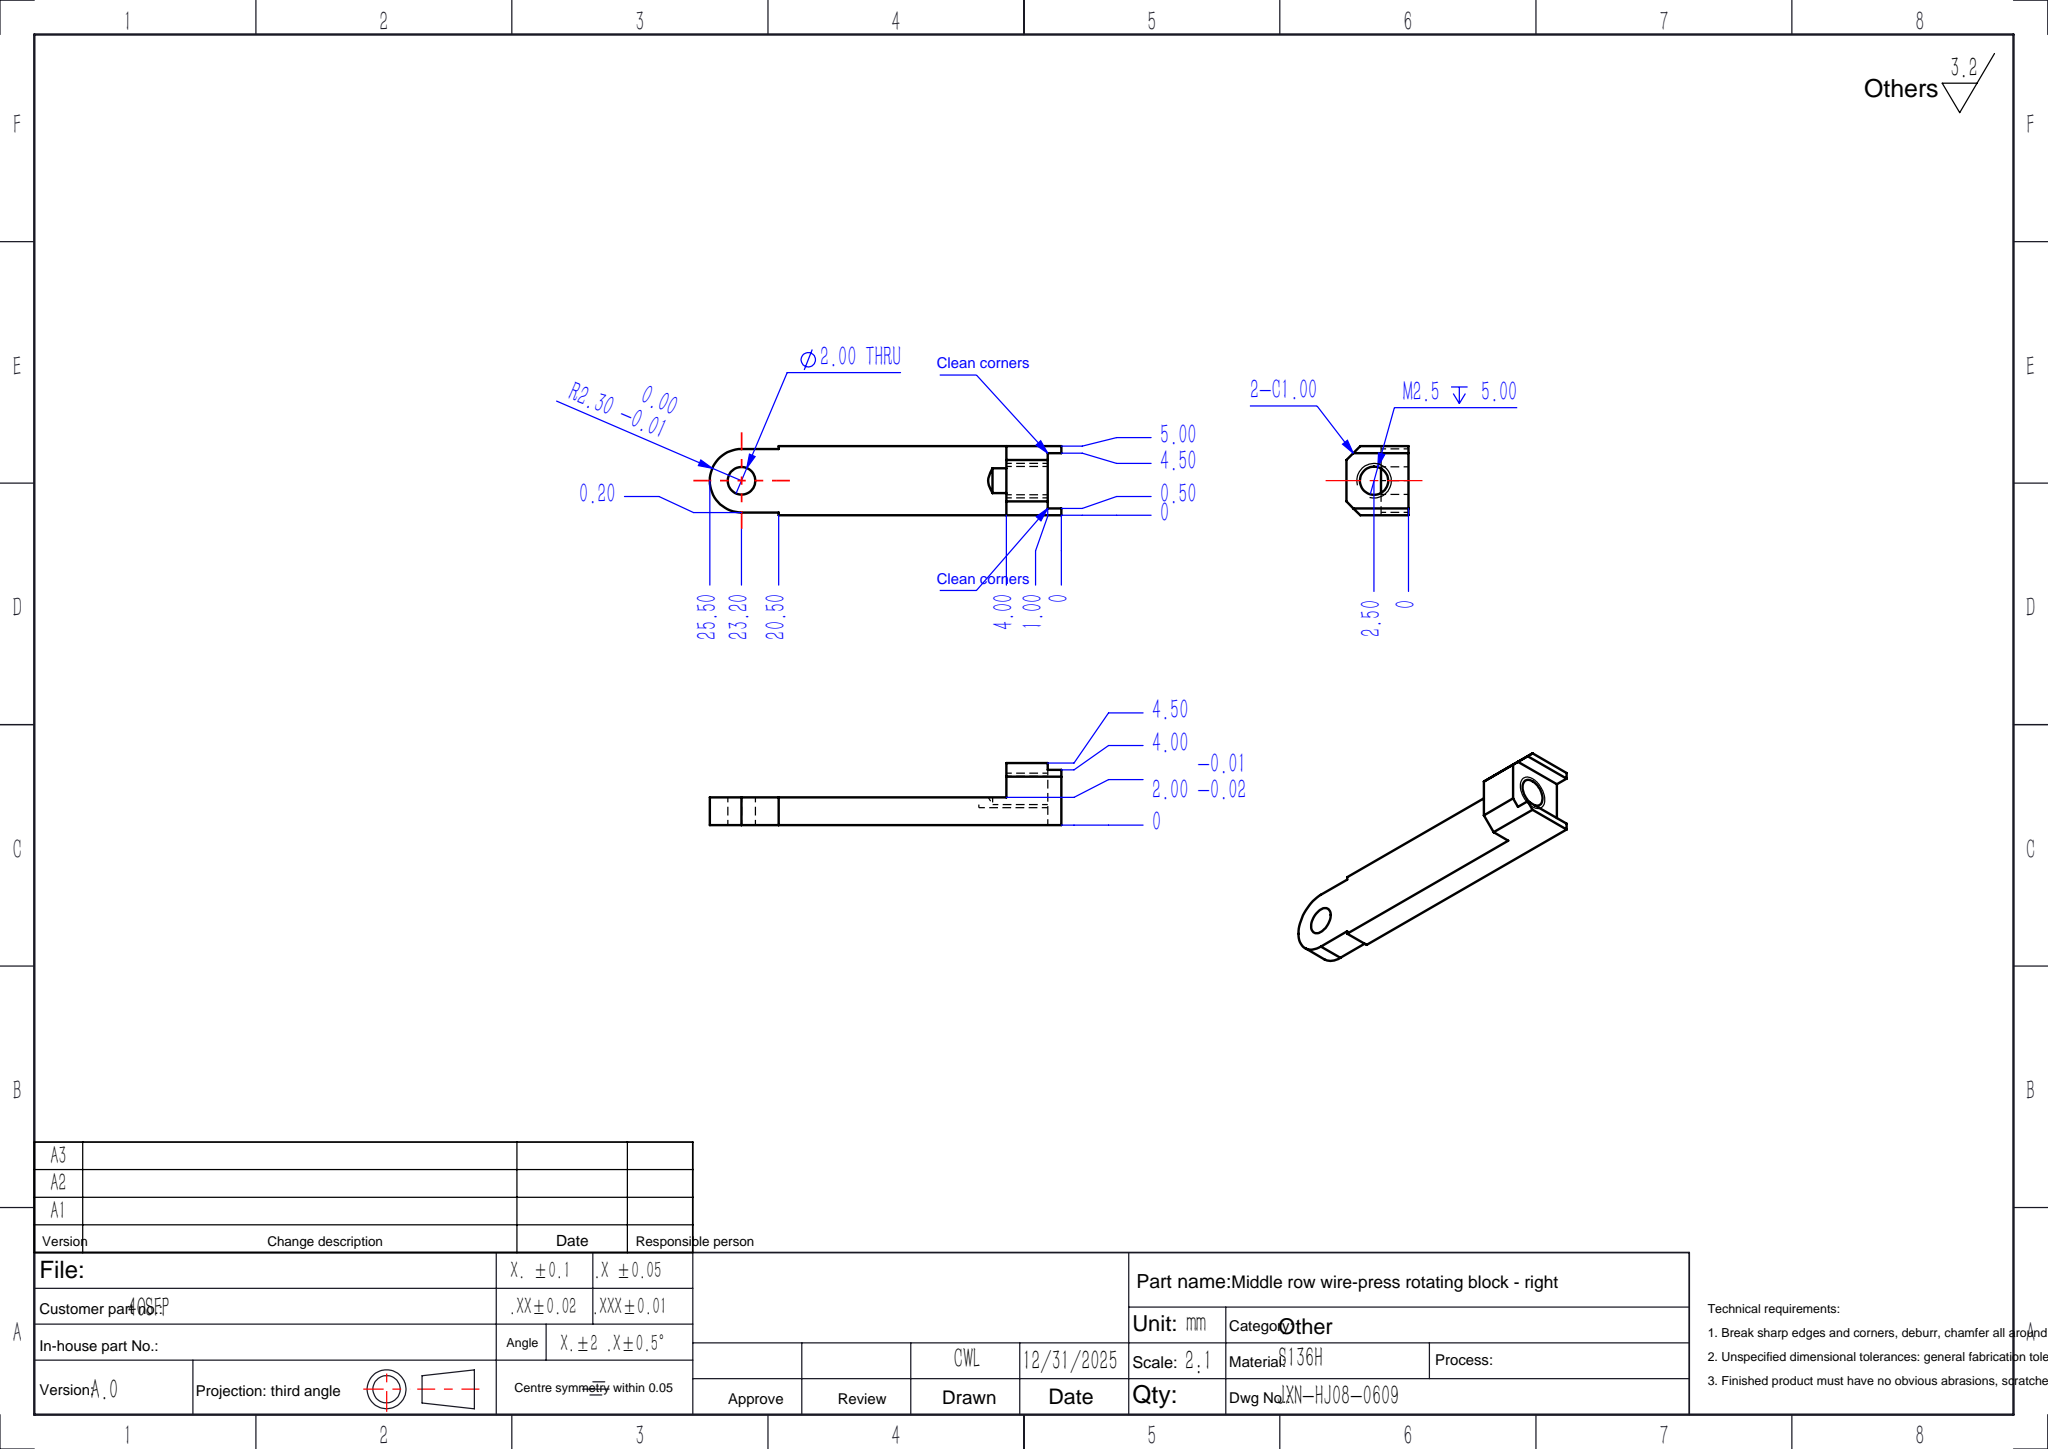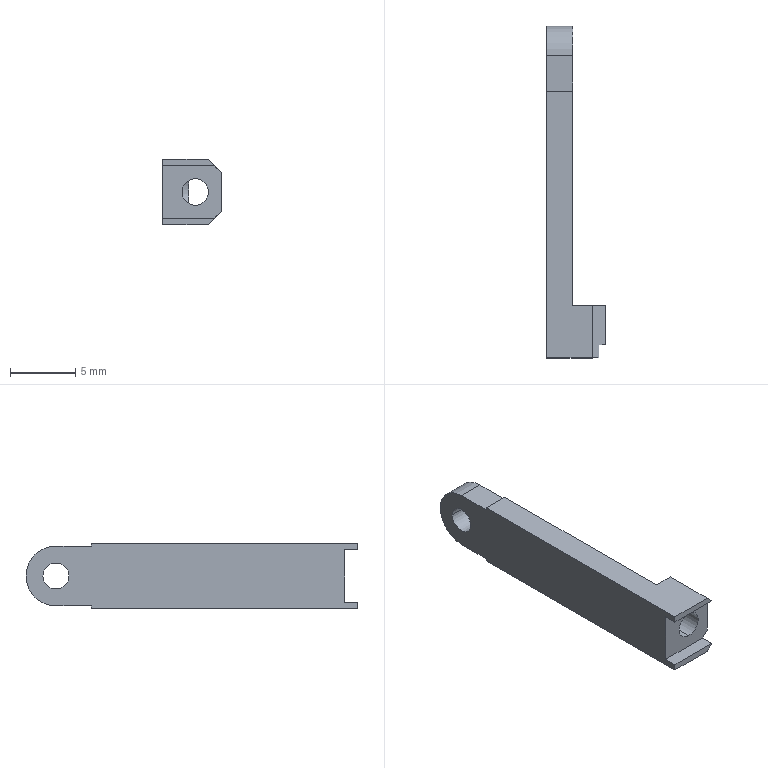Part | SolidWorks | features ICE 4, Chamfer 1, Extrusion 1, Fillet 1, HoleWzd 1 | 1 solid | 24 faces | box 4.5 x 25.5 x 5 mm | volume 257.777 mm3 | plane 17 | cylinder 6 | cone 1 | commonest cylinder face diameters 2 x2 2.05 x2 4.6 x2
STEP:
#1=CARTESIAN_POINT('',(2.5,-21.5,-1.475));
#2=VERTEX_POINT('',#1);
#3=CARTESIAN_POINT('',(2.,-21.5,-1.605));
#4=VERTEX_POINT('',#3);
#5=CARTESIAN_POINT('',(2.5,-21.5,-2.5));
#6=DIRECTION('',(0.,-1.,0.));
#7=DIRECTION('',(0.,0.,-1.));
#8=AXIS2_PLACEMENT_3D('',#5,#6,#7);
#9=CIRCLE('',#8,1.025);
#10=EDGE_CURVE('',#2,#4,#9,.T.);
#11=ORIENTED_EDGE('',*,*,#10,.F.);
#12=CARTESIAN_POINT('',(2.5,-24.5,-1.475));
#13=VERTEX_POINT('',#12);
#14=CARTESIAN_POINT('',(2.5,-24.5,-1.475));
#15=DIRECTION('',(0.,-1.,0.));
#16=VECTOR('',#15,1000.);
#17=LINE('',#14,#16);
#18=EDGE_CURVE('',#2,#13,#17,.T.);
#19=ORIENTED_EDGE('',*,*,#18,.T.);
#20=CARTESIAN_POINT('',(2.5,-24.5,-3.525));
#21=VERTEX_POINT('',#20);
#22=CARTESIAN_POINT('',(2.5,-24.5,-2.5));
#23=DIRECTION('',(0.,-1.,0.));
#24=DIRECTION('',(0.,0.,-1.));
#25=AXIS2_PLACEMENT_3D('',#22,#23,#24);
#26=CIRCLE('',#25,1.025);
#27=EDGE_CURVE('',#13,#21,#26,.T.);
#28=ORIENTED_EDGE('',*,*,#27,.T.);
#29=CARTESIAN_POINT('',(2.5,-21.5,-3.525));
#30=VERTEX_POINT('',#29);
#31=CARTESIAN_POINT('',(2.5,-24.5,-3.525));
#32=DIRECTION('',(0.,-1.,0.));
#33=VECTOR('',#32,1000.);
#34=LINE('',#31,#33);
#35=EDGE_CURVE('',#30,#21,#34,.T.);
#36=ORIENTED_EDGE('',*,*,#35,.F.);
#37=CARTESIAN_POINT('',(2.,-21.5,-3.395));
#38=VERTEX_POINT('',#37);
#39=CARTESIAN_POINT('',(2.5,-21.5,-2.5));
#40=DIRECTION('',(0.,-1.,0.));
#41=DIRECTION('',(0.,0.,-1.));
#42=AXIS2_PLACEMENT_3D('',#39,#40,#41);
#43=CIRCLE('',#42,1.025);
#44=EDGE_CURVE('',#38,#30,#43,.T.);
#45=ORIENTED_EDGE('',*,*,#44,.F.);
#46=CARTESIAN_POINT('',(2.,-20.5,-3.395));
#47=VERTEX_POINT('',#46);
#48=CARTESIAN_POINT('',(2.,-24.5,-3.395));
#49=DIRECTION('',(0.,-1.,0.));
#50=VECTOR('',#49,1000.);
#51=LINE('',#48,#50);
#52=EDGE_CURVE('',#47,#38,#51,.T.);
#53=ORIENTED_EDGE('',*,*,#52,.F.);
#54=CARTESIAN_POINT('',(2.,-20.5,-1.605));
#55=VERTEX_POINT('',#54);
#56=CARTESIAN_POINT('',(2.5,-20.5,-2.5));
#57=DIRECTION('',(0.,-1.,0.));
#58=DIRECTION('',(0.,0.,-1.));
#59=AXIS2_PLACEMENT_3D('',#56,#57,#58);
#60=CIRCLE('',#59,1.025);
#61=EDGE_CURVE('',#55,#47,#60,.T.);
#62=ORIENTED_EDGE('',*,*,#61,.F.);
#63=CARTESIAN_POINT('',(2.,-24.5,-1.605));
#64=DIRECTION('',(0.,1.,0.));
#65=VECTOR('',#64,1000.);
#66=LINE('',#63,#65);
#67=EDGE_CURVE('',#4,#55,#66,.T.);
#68=ORIENTED_EDGE('',*,*,#67,.F.);
#69=EDGE_LOOP('',(#11,#19,#28,#36,#45,#53,#62,#68));
#70=FACE_OUTER_BOUND('',#69,.T.);
#71=CARTESIAN_POINT('',(2.5,-24.5,-2.5));
#72=DIRECTION('',(0.,-1.,0.));
#73=DIRECTION('',(0.,0.,-1.));
#74=AXIS2_PLACEMENT_3D('',#71,#72,#73);
#75=CYLINDRICAL_SURFACE('',#74,1.025);
#76=ADVANCED_FACE('',(#70),#75,.F.);
#77=CARTESIAN_POINT('',(2.,-3.3,-2.5));
#78=VERTEX_POINT('',#77);
#79=CARTESIAN_POINT('',(2.,-1.3,-2.5));
#80=VERTEX_POINT('',#79);
#81=CARTESIAN_POINT('',(2.,-2.3,-2.5));
#82=DIRECTION('',(1.,0.,0.));
#83=DIRECTION('',(0.,-1.,0.));
#84=AXIS2_PLACEMENT_3D('',#81,#82,#83);
#85=CIRCLE('',#84,1.);
#86=EDGE_CURVE('',#78,#80,#85,.T.);
#87=ORIENTED_EDGE('',*,*,#86,.T.);
#88=CARTESIAN_POINT('',(0.,-1.3,-2.5));
#89=VERTEX_POINT('',#88);
#90=CARTESIAN_POINT('',(4.5,-1.3,-2.5));
#91=DIRECTION('',(-1.,0.,0.));
#92=VECTOR('',#91,1000.);
#93=LINE('',#90,#92);
#94=EDGE_CURVE('',#80,#89,#93,.T.);
#95=ORIENTED_EDGE('',*,*,#94,.T.);
#96=CARTESIAN_POINT('',(0.,-3.3,-2.5));
#97=VERTEX_POINT('',#96);
#98=CARTESIAN_POINT('',(0.,-2.3,-2.5));
#99=DIRECTION('',(-1.,0.,0.));
#100=DIRECTION('',(0.,-1.,0.));
#101=AXIS2_PLACEMENT_3D('',#98,#99,#100);
#102=CIRCLE('',#101,1.);
#103=EDGE_CURVE('',#89,#97,#102,.T.);
#104=ORIENTED_EDGE('',*,*,#103,.T.);
#105=CARTESIAN_POINT('',(4.5,-3.3,-2.5));
#106=DIRECTION('',(-1.,0.,0.));
#107=VECTOR('',#106,1000.);
#108=LINE('',#105,#107);
#109=EDGE_CURVE('',#78,#97,#108,.T.);
#110=ORIENTED_EDGE('',*,*,#109,.F.);
#111=EDGE_LOOP('',(#87,#95,#104,#110));
#112=FACE_OUTER_BOUND('',#111,.T.);
#113=CARTESIAN_POINT('',(4.5,-2.3,-2.5));
#114=DIRECTION('',(-1.,0.,0.));
#115=DIRECTION('',(0.,-1.,0.));
#116=AXIS2_PLACEMENT_3D('',#113,#114,#115);
#117=CYLINDRICAL_SURFACE('',#116,1.);
#118=ADVANCED_FACE('',(#112),#117,.F.);
#119=CARTESIAN_POINT('',(4.,-25.5,-0.5));
#120=VERTEX_POINT('',#119);
#121=CARTESIAN_POINT('',(0.,-25.5,-0.5));
#122=VERTEX_POINT('',#121);
#123=CARTESIAN_POINT('',(4.5,-25.5,-0.5));
#124=DIRECTION('',(-1.,0.,0.));
#125=VECTOR('',#124,1000.);
#126=LINE('',#123,#125);
#127=EDGE_CURVE('',#120,#122,#126,.T.);
#128=ORIENTED_EDGE('',*,*,#127,.F.);
#129=CARTESIAN_POINT('',(3.5,-25.5,0.));
#130=VERTEX_POINT('',#129);
#131=CARTESIAN_POINT('',(4.25,-25.5,-0.75));
#132=DIRECTION('',(-0.7071,0.,0.7071));
#133=VECTOR('',#132,1000.);
#134=LINE('',#131,#133);
#135=EDGE_CURVE('',#120,#130,#134,.T.);
#136=ORIENTED_EDGE('',*,*,#135,.T.);
#137=CARTESIAN_POINT('',(0.,-25.5,0.));
#138=VERTEX_POINT('',#137);
#139=CARTESIAN_POINT('',(0.,-25.5,0.));
#140=DIRECTION('',(1.,0.,0.));
#141=VECTOR('',#140,1000.);
#142=LINE('',#139,#141);
#143=EDGE_CURVE('',#138,#130,#142,.T.);
#144=ORIENTED_EDGE('',*,*,#143,.F.);
#145=CARTESIAN_POINT('',(0.,-25.5,-5.));
#146=DIRECTION('',(0.,0.,1.));
#147=VECTOR('',#146,1000.);
#148=LINE('',#145,#147);
#149=EDGE_CURVE('',#122,#138,#148,.T.);
#150=ORIENTED_EDGE('',*,*,#149,.F.);
#151=EDGE_LOOP('',(#128,#136,#144,#150));
#152=FACE_OUTER_BOUND('',#151,.T.);
#153=CARTESIAN_POINT('',(0.,-25.5,-5.));
#154=DIRECTION('',(0.,-1.,0.));
#155=DIRECTION('',(0.,0.,-1.));
#156=AXIS2_PLACEMENT_3D('',#153,#154,#155);
#157=PLANE('',#156);
#158=ADVANCED_FACE('',(#152),#157,.T.);
#159=CARTESIAN_POINT('',(0.,-24.5,-0.5));
#160=VERTEX_POINT('',#159);
#161=CARTESIAN_POINT('',(0.,-25.5,-0.5));
#162=DIRECTION('',(0.,1.,0.));
#163=VECTOR('',#162,1000.);
#164=LINE('',#161,#163);
#165=EDGE_CURVE('',#122,#160,#164,.T.);
#166=ORIENTED_EDGE('',*,*,#165,.F.);
#167=ORIENTED_EDGE('',*,*,#149,.T.);
#168=CARTESIAN_POINT('',(0.,-5.,0.));
#169=VERTEX_POINT('',#168);
#170=CARTESIAN_POINT('',(0.,0.,0.));
#171=DIRECTION('',(0.,-1.,0.));
#172=VECTOR('',#171,1000.);
#173=LINE('',#170,#172);
#174=EDGE_CURVE('',#169,#138,#173,.T.);
#175=ORIENTED_EDGE('',*,*,#174,.F.);
#176=CARTESIAN_POINT('',(0.,-5.,-0.2));
#177=VERTEX_POINT('',#176);
#178=CARTESIAN_POINT('',(0.,-5.,0.));
#179=DIRECTION('',(0.,0.,1.));
#180=VECTOR('',#179,1000.);
#181=LINE('',#178,#180);
#182=EDGE_CURVE('',#177,#169,#181,.T.);
#183=ORIENTED_EDGE('',*,*,#182,.F.);
#184=CARTESIAN_POINT('',(0.,-2.3,-0.2));
#185=VERTEX_POINT('',#184);
#186=CARTESIAN_POINT('',(0.,0.,-0.2));
#187=DIRECTION('',(0.,-1.,0.));
#188=VECTOR('',#187,1000.);
#189=LINE('',#186,#188);
#190=EDGE_CURVE('',#185,#177,#189,.T.);
#191=ORIENTED_EDGE('',*,*,#190,.F.);
#192=CARTESIAN_POINT('',(0.,0.,-2.5));
#193=VERTEX_POINT('',#192);
#194=CARTESIAN_POINT('',(0.,-2.3,-2.5));
#195=DIRECTION('',(-1.,0.,0.));
#196=DIRECTION('',(0.,-1.,0.));
#197=AXIS2_PLACEMENT_3D('',#194,#195,#196);
#198=CIRCLE('',#197,2.3);
#199=EDGE_CURVE('',#185,#193,#198,.T.);
#200=ORIENTED_EDGE('',*,*,#199,.T.);
#201=CARTESIAN_POINT('',(0.,-2.3,-4.8));
#202=VERTEX_POINT('',#201);
#203=CARTESIAN_POINT('',(0.,-2.3,-2.5));
#204=DIRECTION('',(-1.,0.,0.));
#205=DIRECTION('',(0.,-1.,0.));
#206=AXIS2_PLACEMENT_3D('',#203,#204,#205);
#207=CIRCLE('',#206,2.3);
#208=EDGE_CURVE('',#193,#202,#207,.T.);
#209=ORIENTED_EDGE('',*,*,#208,.T.);
#210=CARTESIAN_POINT('',(0.,-5.,-4.8));
#211=VERTEX_POINT('',#210);
#212=CARTESIAN_POINT('',(0.,0.,-4.8));
#213=DIRECTION('',(0.,1.,0.));
#214=VECTOR('',#213,1000.);
#215=LINE('',#212,#214);
#216=EDGE_CURVE('',#211,#202,#215,.T.);
#217=ORIENTED_EDGE('',*,*,#216,.F.);
#218=CARTESIAN_POINT('',(0.,-5.,-5.));
#219=VERTEX_POINT('',#218);
#220=CARTESIAN_POINT('',(0.,-5.,-5.));
#221=DIRECTION('',(0.,0.,1.));
#222=VECTOR('',#221,1000.);
#223=LINE('',#220,#222);
#224=EDGE_CURVE('',#219,#211,#223,.T.);
#225=ORIENTED_EDGE('',*,*,#224,.F.);
#226=CARTESIAN_POINT('',(0.,-25.5,-5.));
#227=VERTEX_POINT('',#226);
#228=CARTESIAN_POINT('',(0.,0.,-5.));
#229=DIRECTION('',(0.,-1.,0.));
#230=VECTOR('',#229,1000.);
#231=LINE('',#228,#230);
#232=EDGE_CURVE('',#219,#227,#231,.T.);
#233=ORIENTED_EDGE('',*,*,#232,.T.);
#234=CARTESIAN_POINT('',(0.,-25.5,-4.5));
#235=VERTEX_POINT('',#234);
#236=CARTESIAN_POINT('',(0.,-25.5,-5.));
#237=DIRECTION('',(0.,0.,1.));
#238=VECTOR('',#237,1000.);
#239=LINE('',#236,#238);
#240=EDGE_CURVE('',#227,#235,#239,.T.);
#241=ORIENTED_EDGE('',*,*,#240,.T.);
#242=CARTESIAN_POINT('',(0.,-24.5,-4.5));
#243=VERTEX_POINT('',#242);
#244=CARTESIAN_POINT('',(0.,-25.5,-4.5));
#245=DIRECTION('',(0.,-1.,0.));
#246=VECTOR('',#245,1000.);
#247=LINE('',#244,#246);
#248=EDGE_CURVE('',#243,#235,#247,.T.);
#249=ORIENTED_EDGE('',*,*,#248,.F.);
#250=CARTESIAN_POINT('',(0.,-24.5,-0.5));
#251=DIRECTION('',(0.,0.,-1.));
#252=VECTOR('',#251,1000.);
#253=LINE('',#250,#252);
#254=EDGE_CURVE('',#160,#243,#253,.T.);
#255=ORIENTED_EDGE('',*,*,#254,.F.);
#256=EDGE_LOOP('',(#166,#167,#175,#183,#191,#200,#209,#217,#225,#233,#241,#249,#255));
#257=FACE_OUTER_BOUND('',#256,.T.);
#258=CARTESIAN_POINT('',(0.,-2.3,-2.5));
#259=DIRECTION('',(-1.,0.,0.));
#260=DIRECTION('',(0.,-1.,0.));
#261=AXIS2_PLACEMENT_3D('',#258,#259,#260);
#262=CIRCLE('',#261,1.);
#263=EDGE_CURVE('',#97,#89,#262,.T.);
#264=ORIENTED_EDGE('',*,*,#263,.F.);
#265=ORIENTED_EDGE('',*,*,#103,.F.);
#266=EDGE_LOOP('',(#264,#265));
#267=FACE_BOUND('',#266,.T.);
#268=CARTESIAN_POINT('',(0.,0.,-5.));
#269=DIRECTION('',(-1.,0.,0.));
#270=DIRECTION('',(0.,-1.,0.));
#271=AXIS2_PLACEMENT_3D('',#268,#269,#270);
#272=PLANE('',#271);
#273=ADVANCED_FACE('',(#257,#267),#272,.T.);
#274=CARTESIAN_POINT('',(4.5,-21.5,-4.));
#275=VERTEX_POINT('',#274);
#276=CARTESIAN_POINT('',(4.5,-21.5,-1.));
#277=VERTEX_POINT('',#276);
#278=CARTESIAN_POINT('',(4.5,-21.5,-5.));
#279=DIRECTION('',(0.,0.,1.));
#280=VECTOR('',#279,1000.);
#281=LINE('',#278,#280);
#282=EDGE_CURVE('',#275,#277,#281,.T.);
#283=ORIENTED_EDGE('',*,*,#282,.T.);
#284=CARTESIAN_POINT('',(4.5,-24.5,-1.));
#285=VERTEX_POINT('',#284);
#286=CARTESIAN_POINT('',(4.5,0.,-1.));
#287=DIRECTION('',(0.,-1.,0.));
#288=VECTOR('',#287,1000.);
#289=LINE('',#286,#288);
#290=EDGE_CURVE('',#277,#285,#289,.T.);
#291=ORIENTED_EDGE('',*,*,#290,.T.);
#292=CARTESIAN_POINT('',(4.5,-24.5,-4.));
#293=VERTEX_POINT('',#292);
#294=CARTESIAN_POINT('',(4.5,-24.5,-0.5));
#295=DIRECTION('',(0.,0.,-1.));
#296=VECTOR('',#295,1000.);
#297=LINE('',#294,#296);
#298=EDGE_CURVE('',#285,#293,#297,.T.);
#299=ORIENTED_EDGE('',*,*,#298,.T.);
#300=CARTESIAN_POINT('',(4.5,-21.5,-4.));
#301=DIRECTION('',(0.,1.,0.));
#302=VECTOR('',#301,1000.);
#303=LINE('',#300,#302);
#304=EDGE_CURVE('',#293,#275,#303,.T.);
#305=ORIENTED_EDGE('',*,*,#304,.T.);
#306=EDGE_LOOP('',(#283,#291,#299,#305));
#307=FACE_OUTER_BOUND('',#306,.T.);
#308=CARTESIAN_POINT('',(4.5,0.,-5.));
#309=DIRECTION('',(1.,0.,0.));
#310=DIRECTION('',(0.,1.,0.));
#311=AXIS2_PLACEMENT_3D('',#308,#309,#310);
#312=PLANE('',#311);
#313=ADVANCED_FACE('',(#307),#312,.T.);
#314=CARTESIAN_POINT('',(3.5,-25.5,-5.));
#315=VERTEX_POINT('',#314);
#316=CARTESIAN_POINT('',(0.,-25.5,-5.));
#317=DIRECTION('',(1.,0.,0.));
#318=VECTOR('',#317,1000.);
#319=LINE('',#316,#318);
#320=EDGE_CURVE('',#227,#315,#319,.T.);
#321=ORIENTED_EDGE('',*,*,#320,.T.);
#322=CARTESIAN_POINT('',(4.,-25.5,-4.5));
#323=VERTEX_POINT('',#322);
#324=CARTESIAN_POINT('',(1.75,-25.5,-6.75));
#325=DIRECTION('',(0.7071,0.,0.7071));
#326=VECTOR('',#325,1000.);
#327=LINE('',#324,#326);
#328=EDGE_CURVE('',#315,#323,#327,.T.);
#329=ORIENTED_EDGE('',*,*,#328,.T.);
#330=CARTESIAN_POINT('',(4.5,-25.5,-4.5));
#331=DIRECTION('',(-1.,0.,0.));
#332=VECTOR('',#331,1000.);
#333=LINE('',#330,#332);
#334=EDGE_CURVE('',#323,#235,#333,.T.);
#335=ORIENTED_EDGE('',*,*,#334,.T.);
#336=ORIENTED_EDGE('',*,*,#240,.F.);
#337=EDGE_LOOP('',(#321,#329,#335,#336));
#338=FACE_OUTER_BOUND('',#337,.T.);
#339=CARTESIAN_POINT('',(0.,-25.5,-5.));
#340=DIRECTION('',(0.,-1.,0.));
#341=DIRECTION('',(0.,0.,-1.));
#342=AXIS2_PLACEMENT_3D('',#339,#340,#341);
#343=PLANE('',#342);
#344=ADVANCED_FACE('',(#338),#343,.T.);
#345=CARTESIAN_POINT('',(2.,-21.5,-5.));
#346=VERTEX_POINT('',#345);
#347=CARTESIAN_POINT('',(3.5,-21.5,-5.));
#348=VERTEX_POINT('',#347);
#349=CARTESIAN_POINT('',(4.5,-21.5,-5.));
#350=DIRECTION('',(1.,0.,0.));
#351=VECTOR('',#350,1000.);
#352=LINE('',#349,#351);
#353=EDGE_CURVE('',#346,#348,#352,.T.);
#354=ORIENTED_EDGE('',*,*,#353,.T.);
#355=CARTESIAN_POINT('',(3.5,-25.5,-5.));
#356=DIRECTION('',(0.,-1.,0.));
#357=VECTOR('',#356,1000.);
#358=LINE('',#355,#357);
#359=EDGE_CURVE('',#348,#315,#358,.T.);
#360=ORIENTED_EDGE('',*,*,#359,.T.);
#361=ORIENTED_EDGE('',*,*,#320,.F.);
#362=ORIENTED_EDGE('',*,*,#232,.F.);
#363=CARTESIAN_POINT('',(2.,-5.,-5.));
#364=VERTEX_POINT('',#363);
#365=CARTESIAN_POINT('',(4.5,-5.,-5.));
#366=DIRECTION('',(-1.,0.,0.));
#367=VECTOR('',#366,1000.);
#368=LINE('',#365,#367);
#369=EDGE_CURVE('',#364,#219,#368,.T.);
#370=ORIENTED_EDGE('',*,*,#369,.F.);
#371=CARTESIAN_POINT('',(2.,0.,-5.));
#372=DIRECTION('',(0.,-1.,0.));
#373=VECTOR('',#372,1000.);
#374=LINE('',#371,#373);
#375=EDGE_CURVE('',#364,#346,#374,.T.);
#376=ORIENTED_EDGE('',*,*,#375,.T.);
#377=EDGE_LOOP('',(#354,#360,#361,#362,#370,#376));
#378=FACE_OUTER_BOUND('',#377,.T.);
#379=CARTESIAN_POINT('',(0.,0.,-5.));
#380=DIRECTION('',(0.,0.,1.));
#381=DIRECTION('',(1.,0.,0.));
#382=AXIS2_PLACEMENT_3D('',#379,#380,#381);
#383=PLANE('',#382);
#384=ADVANCED_FACE('',(#378),#383,.F.);
#385=ORIENTED_EDGE('',*,*,#143,.T.);
#386=CARTESIAN_POINT('',(3.5,-21.5,0.));
#387=VERTEX_POINT('',#386);
#388=CARTESIAN_POINT('',(3.5,0.,0.));
#389=DIRECTION('',(0.,1.,0.));
#390=VECTOR('',#389,1000.);
#391=LINE('',#388,#390);
#392=EDGE_CURVE('',#130,#387,#391,.T.);
#393=ORIENTED_EDGE('',*,*,#392,.T.);
#394=CARTESIAN_POINT('',(2.,-21.5,0.));
#395=VERTEX_POINT('',#394);
#396=CARTESIAN_POINT('',(4.5,-21.5,0.));
#397=DIRECTION('',(1.,0.,0.));
#398=VECTOR('',#397,1000.);
#399=LINE('',#396,#398);
#400=EDGE_CURVE('',#395,#387,#399,.T.);
#401=ORIENTED_EDGE('',*,*,#400,.F.);
#402=CARTESIAN_POINT('',(2.,-5.,0.));
#403=VERTEX_POINT('',#402);
#404=CARTESIAN_POINT('',(2.,0.,0.));
#405=DIRECTION('',(0.,-1.,0.));
#406=VECTOR('',#405,1000.);
#407=LINE('',#404,#406);
#408=EDGE_CURVE('',#403,#395,#407,.T.);
#409=ORIENTED_EDGE('',*,*,#408,.F.);
#410=CARTESIAN_POINT('',(4.5,-5.,0.));
#411=DIRECTION('',(-1.,0.,0.));
#412=VECTOR('',#411,1000.);
#413=LINE('',#410,#412);
#414=EDGE_CURVE('',#403,#169,#413,.T.);
#415=ORIENTED_EDGE('',*,*,#414,.T.);
#416=ORIENTED_EDGE('',*,*,#174,.T.);
#417=EDGE_LOOP('',(#385,#393,#401,#409,#415,#416));
#418=FACE_OUTER_BOUND('',#417,.T.);
#419=CARTESIAN_POINT('',(0.,0.,0.));
#420=DIRECTION('',(0.,0.,1.));
#421=DIRECTION('',(1.,0.,0.));
#422=AXIS2_PLACEMENT_3D('',#419,#420,#421);
#423=PLANE('',#422);
#424=ADVANCED_FACE('',(#418),#423,.T.);
#425=ORIENTED_EDGE('',*,*,#94,.F.);
#426=CARTESIAN_POINT('',(2.,-2.3,-2.5));
#427=DIRECTION('',(1.,0.,0.));
#428=DIRECTION('',(0.,-1.,0.));
#429=AXIS2_PLACEMENT_3D('',#426,#427,#428);
#430=CIRCLE('',#429,1.);
#431=EDGE_CURVE('',#80,#78,#430,.T.);
#432=ORIENTED_EDGE('',*,*,#431,.T.);
#433=ORIENTED_EDGE('',*,*,#109,.T.);
#434=ORIENTED_EDGE('',*,*,#263,.T.);
#435=EDGE_LOOP('',(#425,#432,#433,#434));
#436=FACE_OUTER_BOUND('',#435,.T.);
#437=CARTESIAN_POINT('',(4.5,-2.3,-2.5));
#438=DIRECTION('',(-1.,0.,0.));
#439=DIRECTION('',(0.,-1.,0.));
#440=AXIS2_PLACEMENT_3D('',#437,#438,#439);
#441=CYLINDRICAL_SURFACE('',#440,1.);
#442=ADVANCED_FACE('',(#436),#441,.F.);
#443=ORIENTED_EDGE('',*,*,#414,.F.);
#444=CARTESIAN_POINT('',(2.,-5.,-0.2));
#445=VERTEX_POINT('',#444);
#446=CARTESIAN_POINT('',(2.,-5.,0.));
#447=DIRECTION('',(0.,0.,-1.));
#448=VECTOR('',#447,1000.);
#449=LINE('',#446,#448);
#450=EDGE_CURVE('',#403,#445,#449,.T.);
#451=ORIENTED_EDGE('',*,*,#450,.T.);
#452=CARTESIAN_POINT('',(4.5,-5.,-0.2));
#453=DIRECTION('',(-1.,0.,0.));
#454=VECTOR('',#453,1000.);
#455=LINE('',#452,#454);
#456=EDGE_CURVE('',#445,#177,#455,.T.);
#457=ORIENTED_EDGE('',*,*,#456,.T.);
#458=ORIENTED_EDGE('',*,*,#182,.T.);
#459=EDGE_LOOP('',(#443,#451,#457,#458));
#460=FACE_OUTER_BOUND('',#459,.T.);
#461=CARTESIAN_POINT('',(4.5,-5.,0.));
#462=DIRECTION('',(0.,-1.,0.));
#463=DIRECTION('',(1.,0.,0.));
#464=AXIS2_PLACEMENT_3D('',#461,#462,#463);
#465=PLANE('',#464);
#466=ADVANCED_FACE('',(#460),#465,.F.);
#467=ORIENTED_EDGE('',*,*,#456,.F.);
#468=CARTESIAN_POINT('',(2.,-2.3,-0.2));
#469=VERTEX_POINT('',#468);
#470=CARTESIAN_POINT('',(2.,0.,-0.2));
#471=DIRECTION('',(0.,1.,0.));
#472=VECTOR('',#471,1000.);
#473=LINE('',#470,#472);
#474=EDGE_CURVE('',#445,#469,#473,.T.);
#475=ORIENTED_EDGE('',*,*,#474,.T.);
#476=CARTESIAN_POINT('',(0.,-2.3,-0.2));
#477=DIRECTION('',(-1.,0.,0.));
#478=VECTOR('',#477,1000.);
#479=LINE('',#476,#478);
#480=EDGE_CURVE('',#469,#185,#479,.T.);
#481=ORIENTED_EDGE('',*,*,#480,.T.);
#482=ORIENTED_EDGE('',*,*,#190,.T.);
#483=EDGE_LOOP('',(#467,#475,#481,#482));
#484=FACE_OUTER_BOUND('',#483,.T.);
#485=CARTESIAN_POINT('',(4.5,0.,-0.2));
#486=DIRECTION('',(0.,0.,-1.));
#487=DIRECTION('',(0.,1.,0.));
#488=AXIS2_PLACEMENT_3D('',#485,#486,#487);
#489=PLANE('',#488);
#490=ADVANCED_FACE('',(#484),#489,.F.);
#491=CARTESIAN_POINT('',(2.,-2.3,-4.8));
#492=VERTEX_POINT('',#491);
#493=CARTESIAN_POINT('',(4.5,-2.3,-4.8));
#494=DIRECTION('',(1.,0.,0.));
#495=VECTOR('',#494,1000.);
#496=LINE('',#493,#495);
#497=EDGE_CURVE('',#202,#492,#496,.T.);
#498=ORIENTED_EDGE('',*,*,#497,.T.);
#499=CARTESIAN_POINT('',(2.,-5.,-4.8));
#500=VERTEX_POINT('',#499);
#501=CARTESIAN_POINT('',(2.,0.,-4.8));
#502=DIRECTION('',(0.,-1.,0.));
#503=VECTOR('',#502,1000.);
#504=LINE('',#501,#503);
#505=EDGE_CURVE('',#492,#500,#504,.T.);
#506=ORIENTED_EDGE('',*,*,#505,.T.);
#507=CARTESIAN_POINT('',(4.5,-5.,-4.8));
#508=DIRECTION('',(-1.,0.,0.));
#509=VECTOR('',#508,1000.);
#510=LINE('',#507,#509);
#511=EDGE_CURVE('',#500,#211,#510,.T.);
#512=ORIENTED_EDGE('',*,*,#511,.T.);
#513=ORIENTED_EDGE('',*,*,#216,.T.);
#514=EDGE_LOOP('',(#498,#506,#512,#513));
#515=FACE_OUTER_BOUND('',#514,.T.);
#516=CARTESIAN_POINT('',(4.5,0.,-4.8));
#517=DIRECTION('',(0.,0.,1.));
#518=DIRECTION('',(0.,-1.,0.));
#519=AXIS2_PLACEMENT_3D('',#516,#517,#518);
#520=PLANE('',#519);
#521=ADVANCED_FACE('',(#515),#520,.F.);
#522=ORIENTED_EDGE('',*,*,#511,.F.);
#523=CARTESIAN_POINT('',(2.,-5.,-5.));
#524=DIRECTION('',(0.,0.,-1.));
#525=VECTOR('',#524,1000.);
#526=LINE('',#523,#525);
#527=EDGE_CURVE('',#500,#364,#526,.T.);
#528=ORIENTED_EDGE('',*,*,#527,.T.);
#529=ORIENTED_EDGE('',*,*,#369,.T.);
#530=ORIENTED_EDGE('',*,*,#224,.T.);
#531=EDGE_LOOP('',(#522,#528,#529,#530));
#532=FACE_OUTER_BOUND('',#531,.T.);
#533=CARTESIAN_POINT('',(4.5,-5.,-5.));
#534=DIRECTION('',(0.,-1.,0.));
#535=DIRECTION('',(1.,0.,0.));
#536=AXIS2_PLACEMENT_3D('',#533,#534,#535);
#537=PLANE('',#536);
#538=ADVANCED_FACE('',(#532),#537,.F.);
#539=CARTESIAN_POINT('',(2.,0.,-2.5));
#540=VERTEX_POINT('',#539);
#541=CARTESIAN_POINT('',(2.,-2.3,-2.5));
#542=DIRECTION('',(1.,0.,0.));
#543=DIRECTION('',(0.,-1.,0.));
#544=AXIS2_PLACEMENT_3D('',#541,#542,#543);
#545=CIRCLE('',#544,2.3);
#546=EDGE_CURVE('',#540,#469,#545,.T.);
#547=ORIENTED_EDGE('',*,*,#546,.F.);
#548=CARTESIAN_POINT('',(4.5,0.,-2.5));
#549=DIRECTION('',(1.,0.,0.));
#550=VECTOR('',#549,1000.);
#551=LINE('',#548,#550);
#552=EDGE_CURVE('',#193,#540,#551,.T.);
#553=ORIENTED_EDGE('',*,*,#552,.F.);
#554=ORIENTED_EDGE('',*,*,#199,.F.);
#555=ORIENTED_EDGE('',*,*,#480,.F.);
#556=EDGE_LOOP('',(#547,#553,#554,#555));
#557=FACE_OUTER_BOUND('',#556,.T.);
#558=CARTESIAN_POINT('',(4.5,-2.3,-2.5));
#559=DIRECTION('',(1.,0.,0.));
#560=DIRECTION('',(0.,0.,-1.));
#561=AXIS2_PLACEMENT_3D('',#558,#559,#560);
#562=CYLINDRICAL_SURFACE('',#561,2.3);
#563=ADVANCED_FACE('',(#557),#562,.T.);
#564=CARTESIAN_POINT('',(2.,-2.3,-2.5));
#565=DIRECTION('',(1.,0.,0.));
#566=DIRECTION('',(0.,-1.,0.));
#567=AXIS2_PLACEMENT_3D('',#564,#565,#566);
#568=CIRCLE('',#567,2.3);
#569=EDGE_CURVE('',#492,#540,#568,.T.);
#570=ORIENTED_EDGE('',*,*,#569,.F.);
#571=ORIENTED_EDGE('',*,*,#497,.F.);
#572=ORIENTED_EDGE('',*,*,#208,.F.);
#573=ORIENTED_EDGE('',*,*,#552,.T.);
#574=EDGE_LOOP('',(#570,#571,#572,#573));
#575=FACE_OUTER_BOUND('',#574,.T.);
#576=CARTESIAN_POINT('',(0.,-2.3,-2.5));
#577=DIRECTION('',(1.,0.,0.));
#578=DIRECTION('',(0.,0.,-1.));
#579=AXIS2_PLACEMENT_3D('',#576,#577,#578);
#580=CYLINDRICAL_SURFACE('',#579,2.3);
#581=ADVANCED_FACE('',(#575),#580,.T.);
#582=CARTESIAN_POINT('',(4.,-24.5,-0.5));
#583=VERTEX_POINT('',#582);
#584=CARTESIAN_POINT('',(4.5,-24.5,-0.5));
#585=DIRECTION('',(-1.,0.,0.));
#586=VECTOR('',#585,1000.);
#587=LINE('',#584,#586);
#588=EDGE_CURVE('',#583,#160,#587,.T.);
#589=ORIENTED_EDGE('',*,*,#588,.F.);
#590=CARTESIAN_POINT('',(4.,0.,-0.5));
#591=DIRECTION('',(0.,-1.,0.));
#592=VECTOR('',#591,1000.);
#593=LINE('',#590,#592);
#594=EDGE_CURVE('',#583,#120,#593,.T.);
#595=ORIENTED_EDGE('',*,*,#594,.T.);
#596=ORIENTED_EDGE('',*,*,#127,.T.);
#597=ORIENTED_EDGE('',*,*,#165,.T.);
#598=EDGE_LOOP('',(#589,#595,#596,#597));
#599=FACE_OUTER_BOUND('',#598,.T.);
#600=CARTESIAN_POINT('',(4.5,-25.5,-0.5));
#601=DIRECTION('',(0.,0.,1.));
#602=DIRECTION('',(0.,-1.,0.));
#603=AXIS2_PLACEMENT_3D('',#600,#601,#602);
#604=PLANE('',#603);
#605=ADVANCED_FACE('',(#599),#604,.F.);
#606=ORIENTED_EDGE('',*,*,#334,.F.);
#607=CARTESIAN_POINT('',(4.,-24.5,-4.5));
#608=VERTEX_POINT('',#607);
#609=CARTESIAN_POINT('',(4.,0.,-4.5));
#610=DIRECTION('',(0.,1.,0.));
#611=VECTOR('',#610,1000.);
#612=LINE('',#609,#611);
#613=EDGE_CURVE('',#323,#608,#612,.T.);
#614=ORIENTED_EDGE('',*,*,#613,.T.);
#615=CARTESIAN_POINT('',(4.5,-24.5,-4.5));
#616=DIRECTION('',(-1.,0.,0.));
#617=VECTOR('',#616,1000.);
#618=LINE('',#615,#617);
#619=EDGE_CURVE('',#608,#243,#618,.T.);
#620=ORIENTED_EDGE('',*,*,#619,.T.);
#621=ORIENTED_EDGE('',*,*,#248,.T.);
#622=EDGE_LOOP('',(#606,#614,#620,#621));
#623=FACE_OUTER_BOUND('',#622,.T.);
#624=CARTESIAN_POINT('',(4.5,-25.5,-4.5));
#625=DIRECTION('',(0.,0.,-1.));
#626=DIRECTION('',(-1.,0.,0.));
#627=AXIS2_PLACEMENT_3D('',#624,#625,#626);
#628=PLANE('',#627);
#629=ADVANCED_FACE('',(#623),#628,.F.);
#630=CARTESIAN_POINT('',(2.5,-24.5,-2.5));
#631=DIRECTION('',(0.,-1.,0.));
#632=DIRECTION('',(0.,0.,-1.));
#633=AXIS2_PLACEMENT_3D('',#630,#631,#632);
#634=CIRCLE('',#633,1.025);
#635=EDGE_CURVE('',#21,#13,#634,.T.);
#636=ORIENTED_EDGE('',*,*,#635,.F.);
#637=ORIENTED_EDGE('',*,*,#27,.F.);
#638=EDGE_LOOP('',(#636,#637));
#639=FACE_BOUND('',#638,.T.);
#640=ORIENTED_EDGE('',*,*,#298,.F.);
#641=CARTESIAN_POINT('',(3.5,-24.5,0.));
#642=DIRECTION('',(-0.7071,0.,0.7071));
#643=VECTOR('',#642,1000.);
#644=LINE('',#641,#643);
#645=EDGE_CURVE('',#285,#583,#644,.T.);
#646=ORIENTED_EDGE('',*,*,#645,.T.);
#647=ORIENTED_EDGE('',*,*,#588,.T.);
#648=ORIENTED_EDGE('',*,*,#254,.T.);
#649=ORIENTED_EDGE('',*,*,#619,.F.);
#650=CARTESIAN_POINT('',(4.5,-24.5,-4.));
#651=DIRECTION('',(0.7071,0.,0.7071));
#652=VECTOR('',#651,1000.);
#653=LINE('',#650,#652);
#654=EDGE_CURVE('',#608,#293,#653,.T.);
#655=ORIENTED_EDGE('',*,*,#654,.T.);
#656=EDGE_LOOP('',(#640,#646,#647,#648,#649,#655));
#657=FACE_OUTER_BOUND('',#656,.T.);
#658=CARTESIAN_POINT('',(4.5,-24.5,-0.5));
#659=DIRECTION('',(0.,1.,0.));
#660=DIRECTION('',(-1.,0.,0.));
#661=AXIS2_PLACEMENT_3D('',#658,#659,#660);
#662=PLANE('',#661);
#663=ADVANCED_FACE('',(#639,#657),#662,.F.);
#664=CARTESIAN_POINT('',(2.,-20.5,-1.605));
#665=CARTESIAN_POINT('',(2.,-20.426,-1.746));
#666=CARTESIAN_POINT('',(2.,-20.355,-1.888));
#667=CARTESIAN_POINT('',(2.,-20.234,-2.182));
#668=CARTESIAN_POINT('',(2.,-20.185,-2.337));
#669=CARTESIAN_POINT('',(2.,-20.184,-2.659));
#670=CARTESIAN_POINT('',(2.,-20.233,-2.814));
#671=CARTESIAN_POINT('',(2.,-20.354,-3.11));
#672=CARTESIAN_POINT('',(2.,-20.426,-3.253));
#673=CARTESIAN_POINT('',(2.,-20.5,-3.395));
#674=B_SPLINE_CURVE_WITH_KNOTS('',3,(#664,#665,#666,#667,#668,#669,#670,#671,#672,#673),.UNSPECIFIED.,.F.,.F.,(4,2,2,2,4),(0.004844,0.005321,0.005798,0.006275,0.006751),.UNSPECIFIED.);
#675=EDGE_CURVE('',#55,#47,#674,.T.);
#676=ORIENTED_EDGE('',*,*,#675,.T.);
#677=ORIENTED_EDGE('',*,*,#52,.T.);
#678=CARTESIAN_POINT('',(2.,-21.5,-5.));
#679=DIRECTION('',(0.,0.,1.));
#680=VECTOR('',#679,1000.);
#681=LINE('',#678,#680);
#682=EDGE_CURVE('',#346,#38,#681,.T.);
#683=ORIENTED_EDGE('',*,*,#682,.F.);
#684=ORIENTED_EDGE('',*,*,#375,.F.);
#685=ORIENTED_EDGE('',*,*,#527,.F.);
#686=ORIENTED_EDGE('',*,*,#505,.F.);
#687=ORIENTED_EDGE('',*,*,#569,.T.);
#688=ORIENTED_EDGE('',*,*,#546,.T.);
#689=ORIENTED_EDGE('',*,*,#474,.F.);
#690=ORIENTED_EDGE('',*,*,#450,.F.);
#691=ORIENTED_EDGE('',*,*,#408,.T.);
#692=CARTESIAN_POINT('',(2.,-21.5,-5.));
#693=DIRECTION('',(0.,0.,1.));
#694=VECTOR('',#693,1000.);
#695=LINE('',#692,#694);
#696=EDGE_CURVE('',#4,#395,#695,.T.);
#697=ORIENTED_EDGE('',*,*,#696,.F.);
#698=ORIENTED_EDGE('',*,*,#67,.T.);
#699=EDGE_LOOP('',(#676,#677,#683,#684,#685,#686,#687,#688,#689,#690,#691,#697,#698));
#700=FACE_OUTER_BOUND('',#699,.T.);
#701=ORIENTED_EDGE('',*,*,#86,.F.);
#702=ORIENTED_EDGE('',*,*,#431,.F.);
#703=EDGE_LOOP('',(#701,#702));
#704=FACE_BOUND('',#703,.T.);
#705=CARTESIAN_POINT('',(2.,0.,-5.));
#706=DIRECTION('',(-1.,0.,0.));
#707=DIRECTION('',(0.,-1.,0.));
#708=AXIS2_PLACEMENT_3D('',#705,#706,#707);
#709=PLANE('',#708);
#710=ADVANCED_FACE('',(#700,#704),#709,.F.);
#711=ORIENTED_EDGE('',*,*,#400,.T.);
#712=CARTESIAN_POINT('',(3.5,-21.5,0.));
#713=DIRECTION('',(0.7071,0.,-0.7071));
#714=VECTOR('',#713,1000.);
#715=LINE('',#712,#714);
#716=EDGE_CURVE('',#387,#277,#715,.T.);
#717=ORIENTED_EDGE('',*,*,#716,.T.);
#718=ORIENTED_EDGE('',*,*,#282,.F.);
#719=CARTESIAN_POINT('',(4.5,-21.5,-4.));
#720=DIRECTION('',(-0.7071,0.,-0.7071));
#721=VECTOR('',#720,1000.);
#722=LINE('',#719,#721);
#723=EDGE_CURVE('',#275,#348,#722,.T.);
#724=ORIENTED_EDGE('',*,*,#723,.T.);
#725=ORIENTED_EDGE('',*,*,#353,.F.);
#726=ORIENTED_EDGE('',*,*,#682,.T.);
#727=ORIENTED_EDGE('',*,*,#44,.T.);
#728=CARTESIAN_POINT('',(2.5,-21.5,-2.5));
#729=DIRECTION('',(0.,-1.,0.));
#730=DIRECTION('',(0.,0.,-1.));
#731=AXIS2_PLACEMENT_3D('',#728,#729,#730);
#732=CIRCLE('',#731,1.025);
#733=EDGE_CURVE('',#30,#2,#732,.T.);
#734=ORIENTED_EDGE('',*,*,#733,.T.);
#735=ORIENTED_EDGE('',*,*,#10,.T.);
#736=ORIENTED_EDGE('',*,*,#696,.T.);
#737=EDGE_LOOP('',(#711,#717,#718,#724,#725,#726,#727,#734,#735,#736));
#738=FACE_OUTER_BOUND('',#737,.T.);
#739=CARTESIAN_POINT('',(4.5,-21.5,-5.));
#740=DIRECTION('',(0.,-1.,0.));
#741=DIRECTION('',(0.,0.,-1.));
#742=AXIS2_PLACEMENT_3D('',#739,#740,#741);
#743=PLANE('',#742);
#744=ADVANCED_FACE('',(#738),#743,.F.);
#745=ORIENTED_EDGE('',*,*,#18,.F.);
#746=ORIENTED_EDGE('',*,*,#733,.F.);
#747=ORIENTED_EDGE('',*,*,#35,.T.);
#748=ORIENTED_EDGE('',*,*,#635,.T.);
#749=EDGE_LOOP('',(#745,#746,#747,#748));
#750=FACE_OUTER_BOUND('',#749,.T.);
#751=CARTESIAN_POINT('',(2.5,-24.5,-2.5));
#752=DIRECTION('',(0.,-1.,0.));
#753=DIRECTION('',(0.,0.,-1.));
#754=AXIS2_PLACEMENT_3D('',#751,#752,#753);
#755=CYLINDRICAL_SURFACE('',#754,1.025);
#756=ADVANCED_FACE('',(#750),#755,.F.);
#757=ORIENTED_EDGE('',*,*,#61,.T.);
#758=ORIENTED_EDGE('',*,*,#675,.F.);
#759=EDGE_LOOP('',(#757,#758));
#760=FACE_OUTER_BOUND('',#759,.T.);
#761=CARTESIAN_POINT('',(2.5,-20.5,-2.5));
#762=DIRECTION('',(0.,-1.,0.));
#763=DIRECTION('',(0.,0.,-1.));
#764=AXIS2_PLACEMENT_3D('',#761,#762,#763);
#765=CONICAL_SURFACE('',#764,1.025,1.03);
#766=ADVANCED_FACE('',(#760),#765,.F.);
#767=ORIENTED_EDGE('',*,*,#645,.F.);
#768=ORIENTED_EDGE('',*,*,#290,.F.);
#769=ORIENTED_EDGE('',*,*,#716,.F.);
#770=ORIENTED_EDGE('',*,*,#392,.F.);
#771=ORIENTED_EDGE('',*,*,#135,.F.);
#772=ORIENTED_EDGE('',*,*,#594,.F.);
#773=EDGE_LOOP('',(#767,#768,#769,#770,#771,#772));
#774=FACE_OUTER_BOUND('',#773,.T.);
#775=CARTESIAN_POINT('',(3.5,0.,0.));
#776=DIRECTION('',(-0.7071,0.,-0.7071));
#777=DIRECTION('',(0.,1.,0.));
#778=AXIS2_PLACEMENT_3D('',#775,#776,#777);
#779=PLANE('',#778);
#780=ADVANCED_FACE('',(#774),#779,.F.);
#781=ORIENTED_EDGE('',*,*,#328,.F.);
#782=ORIENTED_EDGE('',*,*,#359,.F.);
#783=ORIENTED_EDGE('',*,*,#723,.F.);
#784=ORIENTED_EDGE('',*,*,#304,.F.);
#785=ORIENTED_EDGE('',*,*,#654,.F.);
#786=ORIENTED_EDGE('',*,*,#613,.F.);
#787=EDGE_LOOP('',(#781,#782,#783,#784,#785,#786));
#788=FACE_OUTER_BOUND('',#787,.T.);
#789=CARTESIAN_POINT('',(4.5,0.,-4.));
#790=DIRECTION('',(0.7071,0.,-0.7071));
#791=DIRECTION('',(0.,-1.,0.));
#792=AXIS2_PLACEMENT_3D('',#789,#790,#791);
#793=PLANE('',#792);
#794=ADVANCED_FACE('',(#788),#793,.T.);
#795=CLOSED_SHELL('',(#76,#118,#158,#273,#313,#344,#384,#424,#442,#466,#490,#521,#538,#563,#581,#605,#629,#663,#710,#744,#756,#766,#780,#794));
#796=MANIFOLD_SOLID_BREP('',#795);
#797=CARTESIAN_POINT('',(0.,0.,0.));
#798=DIRECTION('',(0.,0.,1.));
#799=DIRECTION('',(1.,0.,0.));
#800=AXIS2_PLACEMENT_3D('',#797,#798,#799);
#801=(LENGTH_UNIT()NAMED_UNIT(*)SI_UNIT(.MILLI.,.METRE.));
#802=UNCERTAINTY_MEASURE_WITH_UNIT(LENGTH_MEASURE(0.00001),#801,'','');
#803=(NAMED_UNIT(*)PLANE_ANGLE_UNIT()SI_UNIT($,.RADIAN.));
#804=(NAMED_UNIT(*)SI_UNIT($,.STERADIAN.)SOLID_ANGLE_UNIT());
#805=(GEOMETRIC_REPRESENTATION_CONTEXT(3)GLOBAL_UNCERTAINTY_ASSIGNED_CONTEXT((#802))GLOBAL_UNIT_ASSIGNED_CONTEXT((#801,#803,#804))REPRESENTATION_CONTEXT('',''));
#806=ADVANCED_BREP_SHAPE_REPRESENTATION('',(#796,#800),#805);